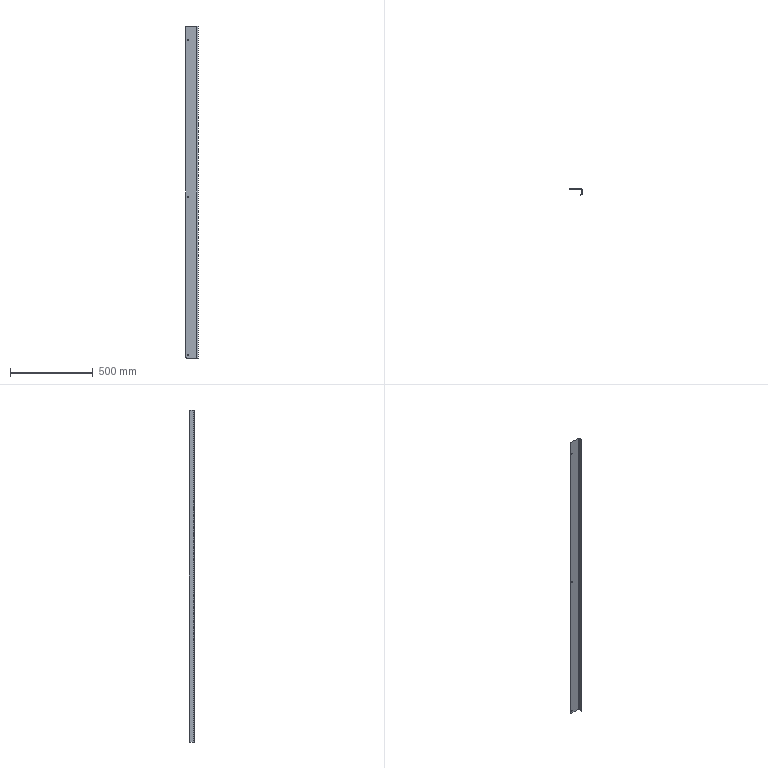Part | STEP file | Guard belt Before lift | 1 solid | 29 faces | box 75 x 33.917 x 2005 mm | volume 340463 mm3 | plane 18 | cylinder 11 | commonest cylinder face diameters 8 x4 6.7 x3 3 x2 6 x2